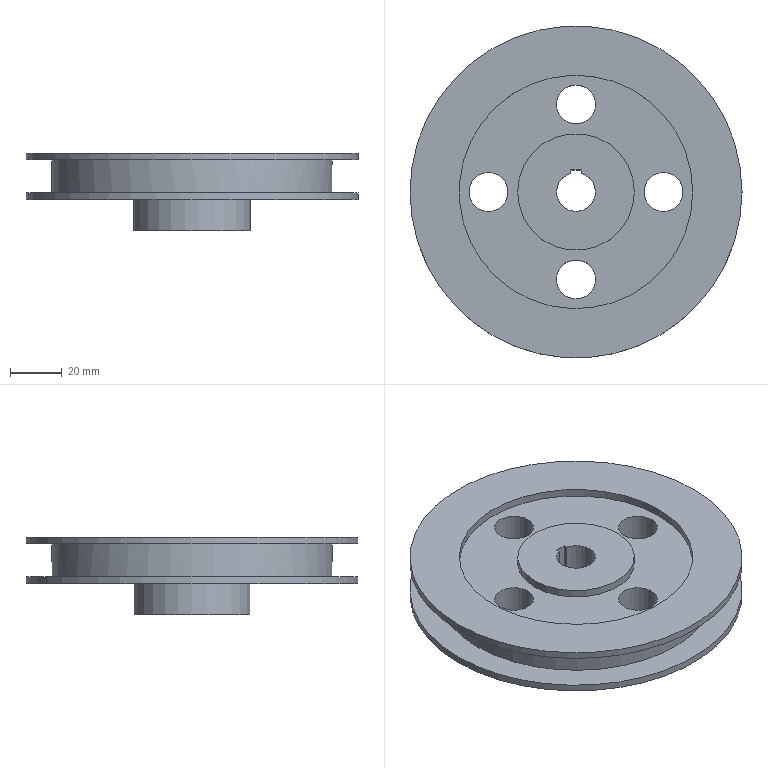Part | STEP file | dadailun | 1 solid | 23 faces | box 128 x 128 x 30 mm | volume 161160 mm3 | cylinder 12 | plane 11 | commonest cylinder face diameters 15 x5 45 x2 90 x2 128 x2 108 x1